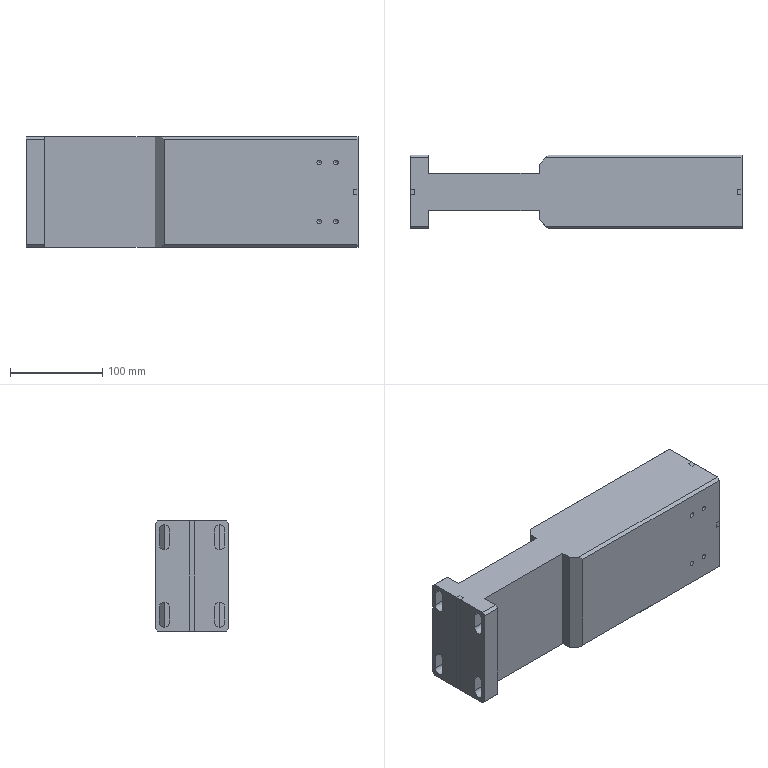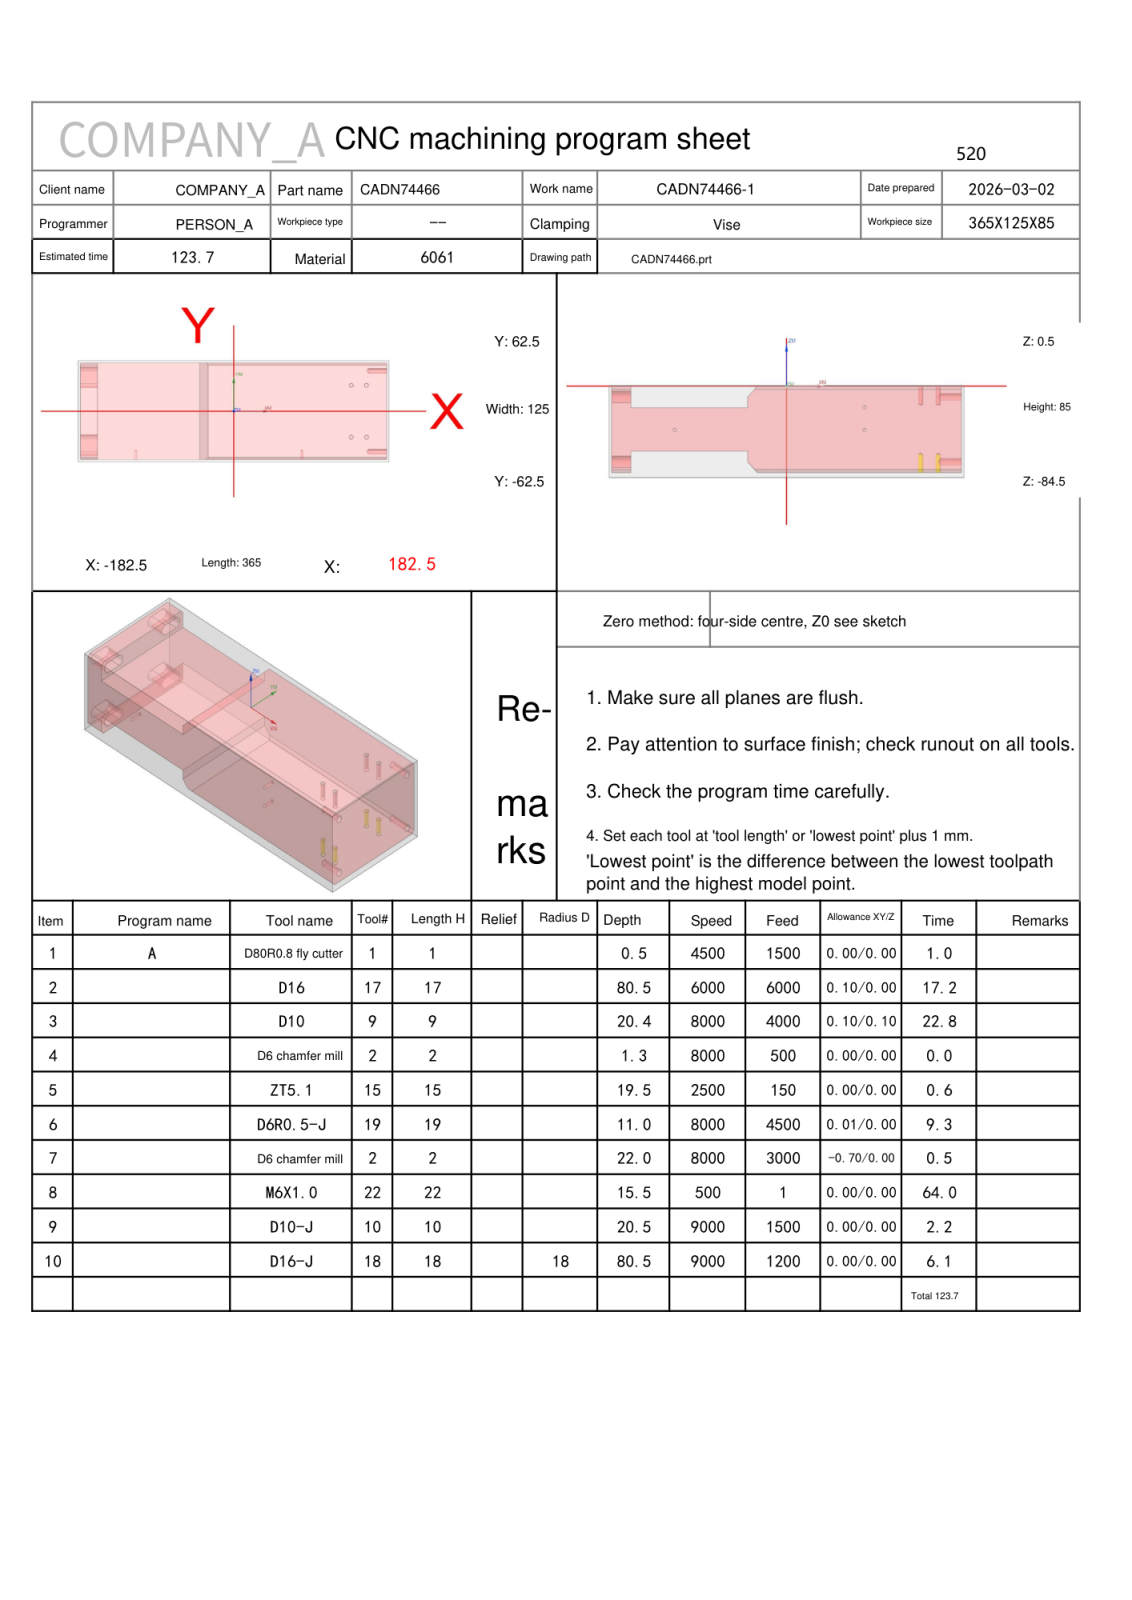NC program | NX | posted by the shop | part box 360 x 80 x 120 mm
Lines 872 to 2006 of 7747:
N3 T09 M06
(D10  D=10. R=0. H=09 ce=0.10 di=0.10)
G00 G90 G54 X-88.269 Y-74.5 M03 S8000
G43 H09 Z10.5
M08
Z.703
G01 Z-.498 F4000.
Y-67.08
G03 X-95.269 Y-60.08 I-7. J0.0
G01 X-147.9
X-154.696
X-154.901 Y-60.079
X-154.986 Y-60.083
X-154.98 Y-59.999
X-154.981 Y-58.427
G03 X-154.9 Y-57.518 I-5.04 J.908
G01 Y-57.497
Y57.497
Y57.518
G03 X-154.981 Y58.427 I-5.121 J0.0
G01 X-154.98 Y59.999
X-154.986 Y60.083
X-154.901 Y60.079
X-154.695 Y60.08
X-45.903
X-45.011
X-38.071
X-38.014 Y60.056
X-35.638 Y57.679
X-35.639 Y53.08
Y-53.08
X-35.638 Y-57.679
X-38.014 Y-60.056
X-38.071 Y-60.08
X-42.639
X-45.088
X-45.903
X-92.255
G02 X-93.068 Y-59.662 I.001 J1.
G01 X-97.471 Y-53.498
G03 X-98.284 Y-53.08 I-.813 J-.582
G01 X-146.902
G02 X-147.9 Y-52.082 I.002 J1.
G01 Y52.082
G02 X-146.902 Y53.08 I1. J-.002
G01 X-45.904
X-45.013
X-43.637
G02 X-42.639 Y52.082 I-.002 J-1.
G01 Y-52.082
G02 X-43.637 Y-53.08 I-1. J.002
G01 X-45.076
X-45.905
X-92.255
G02 X-93.068 Y-52.662 I.001 J1.
G01 X-97.471 Y-46.498
G03 X-98.284 Y-46.08 I-.813 J-.582
G01 X-139.903
G02 X-140.9 Y-45.083 I.003 J1.
G01 Y45.083
G02 X-139.903 Y46.08 I1. J-.003
G01 X-50.636
G02 X-49.639 Y45.083 I-.003 J-1.
G01 Y-45.083
G02 X-50.636 Y-46.08 I-1. J.003
G01 X-92.255
G02 X-93.068 Y-45.662 I.001 J1.
G01 X-97.471 Y-39.498
G03 X-98.284 Y-39.08 I-.813 J-.582
G01 X-132.903
G02 X-133.9 Y-38.083 I.003 J1.
G01 Y38.083
G02 X-132.903 Y39.08 I1. J-.003
G01 X-57.636
G02 X-56.639 Y38.083 I-.003 J-1.
G01 Y-38.083
G02 X-57.636 Y-39.08 I-1. J.003
G01 X-92.255
G02 X-93.068 Y-38.662 I0.0 J1.
G01 X-97.471 Y-32.498
G03 X-98.284 Y-32.08 I-.813 J-.582
G01 X-125.903
G02 X-126.9 Y-31.083 I.003 J1.
G01 Y31.083
G02 X-125.903 Y32.08 I1. J-.003
G01 X-64.636
G02 X-63.639 Y31.083 I-.003 J-1.
G01 Y-31.083
G02 X-64.636 Y-32.08 I-1. J.003
G01 X-92.255
G02 X-93.068 Y-31.662 I0.0 J1.
G01 X-97.471 Y-25.498
G03 X-98.284 Y-25.08 I-.814 J-.582
G01 X-118.904
G02 X-119.9 Y-24.084 I.004 J1.
G01 Y24.084
G02 X-118.904 Y25.08 I1. J-.004
G01 X-71.635
G02 X-70.639 Y24.084 I-.004 J-1.
G01 Y-24.084
G02 X-71.635 Y-25.08 I-1. J.004
G01 X-92.255
G02 X-93.068 Y-24.662 I0.0 J1.
G01 X-97.471 Y-18.498
G03 X-98.284 Y-18.08 I-.814 J-.582
G01 X-111.904
G02 X-112.9 Y-17.084 I.004 J1.
G01 Y17.084
G02 X-111.904 Y18.08 I1. J-.004
G01 X-78.635
G02 X-77.639 Y17.084 I-.004 J-1.
G01 Y-17.084
G02 X-78.635 Y-18.08 I-1. J.004
G01 X-92.255
G02 X-93.068 Y-17.662 I0.0 J1.
G01 X-97.471 Y-11.498
G03 X-98.284 Y-11.08 I-.814 J-.582
G01 X-104.904
G02 X-105.9 Y-10.084 I.004 J1.
G01 Y10.084
G02 X-104.904 Y11.08 I1. J-.004
G01 X-85.635
G02 X-84.639 Y10.084 I-.004 J-1.
G01 Y-10.084
G02 X-85.635 Y-11.08 I-1. J.004
G01 X-92.255
G02 X-93.068 Y-10.662 I0.0 J1.
G01 X-97.502 Y-4.455
G03 X-98.107 Y-4.058 I-.814 J-.582
G02 X-98.9 Y-3.084 I.207 J.978
G01 Y3.084
G02 X-97.904 Y4.08 I1. J-.004
G01 X-92.635
G02 X-91.639 Y3.084 I-.004 J-1.
G01 Y-3.084
G02 X-92.635 Y-4.08 I-1. J.004
G01 X-95.269
X-95.769
G03 X-102.769 Y-11.08 I0.0 J-7.
G01 Z.703
G00 Z3.
G01 X-88.269 Y-74.5 F6000.
G00 Z.205
G01 Z-.995 F4000.
Y-67.08
G03 X-95.269 Y-60.08 I-7. J0.0
G01 X-147.9
X-154.696
X-154.901 Y-60.079
X-154.986 Y-60.083
X-154.98 Y-59.999
X-154.981 Y-58.923
G03 X-154.9 Y-58.016 I-5.04 J.907
G01 Y-57.995
Y57.995
Y58.016
G03 X-154.981 Y58.923 I-5.121 J0.0
G01 X-154.98 Y59.999
X-154.986 Y60.083
X-154.901 Y60.079
X-154.695 Y60.08
X-45.903
X-45.011
X-38.071
X-38.014 Y60.056
X-36.135 Y58.177
X-36.136 Y53.08
Y-53.08
X-36.135 Y-58.177
X-38.014 Y-60.056
X-38.071 Y-60.08
X-43.136
X-45.088
X-45.903
X-92.255
G02 X-93.068 Y-59.662 I.001 J1.
G01 X-97.471 Y-53.498
G03 X-98.284 Y-53.08 I-.813 J-.582
G01 X-146.903
G02 X-147.9 Y-52.083 I.003 J1.
G01 Y52.083
G02 X-146.903 Y53.08 I1. J-.003
G01 X-45.904
X-45.013
X-44.134
G02 X-43.136 Y52.082 I-.003 J-1.
G01 Y-52.082
G02 X-44.134 Y-53.08 I-1. J.003
G01 X-45.076
X-45.905
X-92.255
G02 X-93.068 Y-52.662 I.001 J1.
G01 X-97.471 Y-46.498
G03 X-98.284 Y-46.08 I-.813 J-.582
G01 X-139.903
G02 X-140.9 Y-45.083 I.003 J1.
G01 Y45.083
G02 X-139.903 Y46.08 I1. J-.003
G01 X-51.133
G02 X-50.136 Y45.083 I-.003 J-1.
G01 Y-45.083
G02 X-51.133 Y-46.08 I-1. J.003
G01 X-92.255
G02 X-93.068 Y-45.662 I.001 J1.
G01 X-97.471 Y-39.498
G03 X-98.284 Y-39.08 I-.813 J-.582
G01 X-132.903
G02 X-133.9 Y-38.083 I.003 J1.
G01 Y38.083
G02 X-132.903 Y39.08 I1. J-.003
G01 X-58.133
G02 X-57.136 Y38.083 I-.003 J-1.
G01 Y-38.083
G02 X-58.133 Y-39.08 I-1. J.003
G01 X-92.255
G02 X-93.068 Y-38.662 I0.0 J1.
G01 X-97.471 Y-32.498
G03 X-98.284 Y-32.08 I-.813 J-.582
G01 X-125.904
G02 X-126.9 Y-31.084 I.004 J1.
G01 Y31.084
G02 X-125.904 Y32.08 I1. J-.004
G01 X-65.133
G02 X-64.136 Y31.084 I-.004 J-1.
G01 Y-31.084
G02 X-65.133 Y-32.08 I-1. J.004
G01 X-92.255
G02 X-93.068 Y-31.662 I0.0 J1.
G01 X-97.471 Y-25.498
G03 X-98.284 Y-25.08 I-.814 J-.582
G01 X-118.904
G02 X-119.9 Y-24.084 I.004 J1.
G01 Y24.084
G02 X-118.904 Y25.08 I1. J-.004
G01 X-72.133
G02 X-71.136 Y24.084 I-.004 J-1.
G01 Y-24.084
G02 X-72.133 Y-25.08 I-1. J.004
G01 X-92.255
G02 X-93.068 Y-24.662 I0.0 J1.
G01 X-97.471 Y-18.498
G03 X-98.284 Y-18.08 I-.814 J-.582
G01 X-111.904
G02 X-112.9 Y-17.084 I.004 J1.
G01 Y17.084
G02 X-111.904 Y18.08 I1. J-.004
G01 X-79.133
G02 X-78.136 Y17.084 I-.004 J-1.
G01 Y-17.084
G02 X-79.133 Y-18.08 I-1. J.004
G01 X-92.255
G02 X-93.068 Y-17.662 I0.0 J1.
G01 X-97.471 Y-11.499
G03 X-98.284 Y-11.08 I-.814 J-.581
G01 X-104.904
G02 X-105.9 Y-10.084 I.004 J1.
G01 Y10.084
G02 X-104.904 Y11.08 I1. J-.004
G01 X-86.132
G02 X-85.136 Y10.084 I-.004 J-1.
G01 Y-10.084
G02 X-86.132 Y-11.08 I-1. J.004
G01 X-92.255
G02 X-93.068 Y-10.661 I0.0 J1.
G01 X-97.502 Y-4.455
G03 X-98.107 Y-4.058 I-.814 J-.582
G02 X-98.9 Y-3.084 I.207 J.978
G01 Y3.084
G02 X-97.904 Y4.08 I1. J-.004
G01 X-93.132
G02 X-92.136 Y3.084 I-.004 J-1.
G01 Y-3.084
G02 X-93.132 Y-4.08 I-1. J.004
G01 X-95.269
X-95.769
G03 X-102.769 Y-11.08 I0.0 J-7.
G01 Z.205
G00 Z3.
G01 X-88.269 Y-74.5 F6000.
G00 Z-.293
G01 Z-1.493 F4000.
Y-67.08
G03 X-95.269 Y-60.08 I-7. J0.0
G01 X-147.9
X-154.696
X-154.901 Y-60.079
X-154.986 Y-60.083
X-154.98 Y-59.999
X-154.981 Y-59.419
G03 X-154.9 Y-58.513 I-5.04 J.906
G01 Y-58.492
Y58.492
Y58.513
G03 X-154.981 Y59.419 I-5.121 J0.0
G01 X-154.98 Y59.999
X-154.986 Y60.083
X-154.901 Y60.079
X-154.695 Y60.08
X-45.903
X-45.011
X-38.071
X-38.014 Y60.056
X-36.633 Y58.675
X-36.634 Y53.08
Y-53.08
X-36.633 Y-58.675
X-38.014 Y-60.056
X-38.071 Y-60.08
X-43.634
X-45.088
X-45.903
X-92.255
G02 X-93.068 Y-59.662 I.001 J1.
G01 X-97.471 Y-53.498
G03 X-98.284 Y-53.08 I-.813 J-.582
G01 X-146.903
G02 X-147.9 Y-52.083 I.003 J1.
G01 Y52.083
G02 X-146.903 Y53.08 I1. J-.003
G01 X-45.904
X-45.013
X-44.631
G02 X-43.634 Y52.083 I-.003 J-1.
G01 Y-52.083
G02 X-44.631 Y-53.08 I-1. J.003
G01 X-45.076
X-45.905
X-92.255
G02 X-93.068 Y-52.662 I.001 J1.
G01 X-97.471 Y-46.498
G03 X-98.284 Y-46.08 I-.813 J-.582
G01 X-139.903
G02 X-140.9 Y-45.083 I.003 J1.
G01 Y45.083
G02 X-139.903 Y46.08 I1. J-.003
G01 X-51.631
G02 X-50.634 Y45.083 I-.003 J-1.
G01 Y-45.083
G02 X-51.631 Y-46.08 I-1. J.003
G01 X-92.255
G02 X-93.068 Y-45.662 I.001 J1.
G01 X-97.471 Y-39.498
G03 X-98.284 Y-39.08 I-.813 J-.582
G01 X-132.904
G02 X-133.9 Y-38.084 I.004 J1.
G01 Y38.084
G02 X-132.904 Y39.08 I1. J-.004
G01 X-58.63
G02 X-57.634 Y38.084 I-.004 J-1.
G01 Y-38.084
G02 X-58.63 Y-39.08 I-1. J.004
G01 X-92.255
G02 X-93.068 Y-38.662 I0.0 J1.
G01 X-97.471 Y-32.498
G03 X-98.284 Y-32.08 I-.813 J-.582
G01 X-125.904
G02 X-126.9 Y-31.084 I.004 J1.
G01 Y31.084
G02 X-125.904 Y32.08 I1. J-.004
G01 X-65.63
G02 X-64.634 Y31.084 I-.004 J-1.
G01 Y-31.084
G02 X-65.63 Y-32.08 I-1. J.004
G01 X-92.255
G02 X-93.068 Y-31.662 I0.0 J1.
G01 X-97.471 Y-25.498
G03 X-98.284 Y-25.08 I-.814 J-.582
G01 X-118.904
G02 X-119.9 Y-24.084 I.004 J1.
G01 Y24.084
G02 X-118.904 Y25.08 I1. J-.004
G01 X-72.63
G02 X-71.634 Y24.084 I-.004 J-1.
G01 Y-24.084
G02 X-72.63 Y-25.08 I-1. J.004
G01 X-92.255
G02 X-93.068 Y-24.662 I0.0 J1.
G01 X-97.471 Y-18.498
G03 X-98.284 Y-18.08 I-.814 J-.582
G01 X-111.904
G02 X-112.9 Y-17.084 I.004 J1.
G01 Y17.084
G02 X-111.904 Y18.08 I1. J-.004
G01 X-79.63
G02 X-78.634 Y17.084 I-.004 J-1.
G01 Y-17.084
G02 X-79.63 Y-18.08 I-1. J.004
G01 X-92.255
G02 X-93.068 Y-17.662 I0.0 J1.
G01 X-97.471 Y-11.499
G03 X-98.284 Y-11.08 I-.814 J-.581
G01 X-104.904
G02 X-105.9 Y-10.084 I.004 J1.
G01 Y10.084
G02 X-104.904 Y11.08 I1. J-.004
G01 X-86.63
G02 X-85.634 Y10.084 I-.004 J-1.
G01 Y-10.084
G02 X-86.63 Y-11.08 I-1. J.004
G01 X-92.255
G02 X-93.068 Y-10.661 I0.0 J1.
G01 X-97.502 Y-4.455
G03 X-98.107 Y-4.058 I-.814 J-.582
G02 X-98.9 Y-3.084 I.207 J.978
G01 Y3.084
G02 X-97.904 Y4.08 I1. J-.004
G01 X-93.63
G02 X-92.634 Y3.084 I-.004 J-1.
G01 Y-3.084
G02 X-93.63 Y-4.08 I-1. J.004
G01 X-95.269
X-95.769
G03 X-102.769 Y-11.08 I0.0 J-7.
G01 Z-.293
G00 Z3.
G01 X-88.269 Y-74.5 F6000.
G00 Z-.79
G01 Z-1.99 F4000.
Y-67.08
G03 X-95.269 Y-60.08 I-7. J0.0
G01 X-147.9
X-154.696
X-154.901 Y-60.079
X-154.986 Y-60.083
X-154.98 Y-59.999
Y-59.902
G03 X-154.9 Y-58.996 I-5.055 J.906
G01 Y-58.99
Y58.99
Y59.011
G03 X-154.98 Y59.915 I-5.121 J0.0
G01 Y59.999
X-154.986 Y60.083
X-154.901 Y60.079
X-154.695 Y60.08
X-45.903
X-45.011
X-38.071
X-38.014 Y60.056
X-37.13 Y59.172
X-37.131 Y53.08
Y-53.076
X-37.13 Y-59.172
X-38.014 Y-60.056
X-38.071 Y-60.08
X-44.131
X-45.088
X-45.903
X-92.255
G02 X-93.068 Y-59.662 I.001 J1.
G01 X-97.471 Y-53.498
G03 X-98.284 Y-53.08 I-.813 J-.582
G01 X-146.903
G02 X-147.9 Y-52.083 I.003 J1.
G01 Y52.083
G02 X-146.903 Y53.08 I1. J-.003
G01 X-45.904
X-45.128
G02 X-44.131 Y52.083 I-.003 J-1.
G01 Y-52.083
G02 X-45.128 Y-53.08 I-1. J.003
G01 X-45.905
X-92.255
G02 X-93.068 Y-52.662 I.001 J1.
G01 X-97.471 Y-46.498
G03 X-98.284 Y-46.08 I-.813 J-.582
G01 X-139.903
G02 X-140.9 Y-45.083 I.003 J1.
G01 Y45.083
G02 X-139.903 Y46.08 I1. J-.003
G01 X-52.128
G02 X-51.131 Y45.083 I-.003 J-1.
G01 Y-45.083
G02 X-52.128 Y-46.08 I-1. J.003
G01 X-92.255
G02 X-93.068 Y-45.662 I.001 J1.
G01 X-97.471 Y-39.498
G03 X-98.284 Y-39.08 I-.813 J-.582
G01 X-132.904
G02 X-133.9 Y-38.084 I.004 J1.
G01 Y38.084
G02 X-132.904 Y39.08 I1. J-.004
G01 X-59.128
G02 X-58.131 Y38.084 I-.004 J-1.
G01 Y-38.084
G02 X-59.128 Y-39.08 I-1. J.004
G01 X-92.255
G02 X-93.068 Y-38.662 I0.0 J1.
G01 X-97.471 Y-32.498
G03 X-98.284 Y-32.08 I-.813 J-.582
G01 X-125.904
G02 X-126.9 Y-31.084 I.004 J1.
G01 Y31.084
G02 X-125.904 Y32.08 I1. J-.004
G01 X-66.127
G02 X-65.131 Y31.084 I-.004 J-1.
G01 Y-31.084
G02 X-66.127 Y-32.08 I-1. J.004
G01 X-92.255
G02 X-93.068 Y-31.662 I0.0 J1.
G01 X-97.471 Y-25.498
G03 X-98.284 Y-25.08 I-.813 J-.582
G01 X-118.904
G02 X-119.9 Y-24.084 I.004 J1.
G01 Y24.084
G02 X-118.904 Y25.08 I1. J-.004
G01 X-73.127
G02 X-72.131 Y24.084 I-.004 J-1.
G01 Y-24.084
G02 X-73.127 Y-25.08 I-1. J.004
G01 X-92.255
G02 X-93.068 Y-24.662 I0.0 J1.
G01 X-97.471 Y-18.498
G03 X-98.284 Y-18.08 I-.814 J-.582
G01 X-111.904
G02 X-112.9 Y-17.084 I.004 J1.
G01 Y17.084
G02 X-111.904 Y18.08 I1. J-.004
G01 X-80.127
G02 X-79.131 Y17.084 I-.004 J-1.
G01 Y-17.084
G02 X-80.127 Y-18.08 I-1. J.004
G01 X-92.255
G02 X-93.068 Y-17.662 I0.0 J1.
G01 X-97.471 Y-11.499
G03 X-98.284 Y-11.08 I-.814 J-.581
G01 X-104.904
G02 X-105.9 Y-10.084 I.004 J1.
G01 Y10.084
G02 X-104.904 Y11.08 I1. J-.004
G01 X-87.127
G02 X-86.131 Y10.084 I-.004 J-1.
G01 Y-10.084
G02 X-87.127 Y-11.08 I-1. J.004
G01 X-92.255
G02 X-93.068 Y-10.661 I0.0 J1.
G01 X-97.502 Y-4.455
G03 X-98.107 Y-4.058 I-.814 J-.582
G02 X-98.9 Y-3.084 I.207 J.978
G01 Y3.084
G02 X-97.904 Y4.08 I1. J-.004
G01 X-94.127
G02 X-93.131 Y3.084 I-.004 J-1.
G01 Y-3.084
G02 X-94.127 Y-4.08 I-1. J.004
G01 X-95.269
X-95.769
G03 X-102.769 Y-11.08 I0.0 J-7.
G01 Z-.79
G00 Z3.
G01 X-88.269 Y-74.5 F6000.
G00 Z-1.288
G01 Z-2.488 F4000.
Y-67.08
G03 X-95.269 Y-60.08 I-7. J0.0
G01 X-147.9
X-154.696
X-154.901 Y-60.079
X-154.932 Y-60.072
G03 X-154.9 Y-59.496 I-5.1 J.576
G01 Y-59.487
Y59.487
Y59.496
G03 X-154.932 Y60.072 I-5.133 J0.0
G01 X-154.901 Y60.079
X-154.695 Y60.08
X-45.903
X-45.011
X-38.071
X-38.014 Y60.056
X-37.628 Y59.67
X-37.629 Y53.08
Y-53.076
X-37.628 Y-59.67
X-38.014 Y-60.056
X-38.071 Y-60.08
X-44.629
X-45.088
X-45.903
X-92.255
G02 X-93.068 Y-59.662 I.001 J1.
G01 X-97.471 Y-53.498
G03 X-98.284 Y-53.08 I-.813 J-.582
G01 X-146.903
G02 X-147.9 Y-52.083 I.003 J1.
G01 Y52.083
G02 X-146.903 Y53.08 I1. J-.003
G01 X-45.904
X-45.626
G02 X-44.629 Y52.083 I-.003 J-1.
G01 Y-52.083
G02 X-45.625 Y-53.08 I-1. J.003
G01 X-45.905
X-92.255
G02 X-93.068 Y-52.662 I.001 J1.
G01 X-97.471 Y-46.498
G03 X-98.284 Y-46.08 I-.813 J-.582
G01 X-139.904
G02 X-140.9 Y-45.084 I.004 J1.
G01 Y45.084
G02 X-139.904 Y46.08 I1. J-.004
G01 X-52.625
G02 X-51.629 Y45.084 I-.004 J-1.
G01 Y-45.084
G02 X-52.625 Y-46.08 I-1. J.004
G01 X-92.255
G02 X-93.068 Y-45.662 I.001 J1.
G01 X-97.471 Y-39.498
G03 X-98.284 Y-39.08 I-.813 J-.582
G01 X-132.904
G02 X-133.9 Y-38.084 I.004 J1.
G01 Y38.084
G02 X-132.904 Y39.08 I1. J-.004
G01 X-59.625
G02 X-58.629 Y38.084 I-.004 J-1.
G01 Y-38.084
G02 X-59.625 Y-39.08 I-1. J.004
G01 X-92.255
G02 X-93.068 Y-38.662 I0.0 J1.
G01 X-97.471 Y-32.498
G03 X-98.284 Y-32.08 I-.813 J-.582
G01 X-125.904
G02 X-126.9 Y-31.084 I.004 J1.
G01 Y31.084
G02 X-125.904 Y32.08 I1. J-.004
G01 X-66.625
G02 X-65.629 Y31.084 I-.004 J-1.
G01 Y-31.084
G02 X-66.625 Y-32.08 I-1. J.004
G01 X-92.255
G02 X-93.068 Y-31.662 I0.0 J1.
G01 X-97.471 Y-25.498
G03 X-98.284 Y-25.08 I-.814 J-.582
G01 X-118.904
G02 X-119.9 Y-24.084 I.004 J1.
G01 Y24.084
G02 X-118.904 Y25.08 I1. J-.004
G01 X-73.625
G02 X-72.629 Y24.084 I-.004 J-1.
G01 Y-24.084
G02 X-73.625 Y-25.08 I-1. J.004
G01 X-92.255
G02 X-93.068 Y-24.662 I0.0 J1.
G01 X-97.471 Y-18.498
G03 X-98.284 Y-18.08 I-.814 J-.582
G01 X-111.904
G02 X-112.9 Y-17.084 I.004 J1.
G01 Y17.084
G02 X-111.904 Y18.08 I1. J-.004
G01 X-80.624
G02 X-79.629 Y17.084 I-.004 J-1.
G01 Y-17.084
G02 X-80.624 Y-18.08 I-1. J.004
G01 X-92.255
G02 X-93.068 Y-17.662 I0.0 J1.
G01 X-97.471 Y-11.499
G03 X-98.284 Y-11.08 I-.814 J-.581
G01 X-104.905
G02 X-105.9 Y-10.085 I.005 J1.
G01 Y10.085
G02 X-104.905 Y11.08 I1. J-.005
G01 X-87.624
G02 X-86.629 Y10.085 I-.005 J-1.
G01 Y-10.085
G02 X-87.624 Y-11.08 I-1. J.005
G01 X-92.255
G02 X-93.068 Y-10.661 I0.0 J1.
G01 X-97.502 Y-4.455
G03 X-98.107 Y-4.058 I-.814 J-.582
G02 X-98.9 Y-3.085 I.207 J.978
G01 Y3.085
G02 X-97.905 Y4.08 I1. J-.005
G01 X-94.624
G02 X-93.629 Y3.085 I-.005 J-1.
G01 Y-3.085
G02 X-94.624 Y-4.08 I-1. J.005
G01 X-95.269
X-95.769
G03 X-102.769 Y-11.08 I0.0 J-7.
G01 Z-1.288
G00 Z3.
G01 X-88.269 Y-74.5 F6000.
G00 Z-1.785
G01 Z-2.985 F4000.
Y-67.08
G03 X-95.269 Y-60.08 I-7. J0.0
G01 X-147.9
X-154.696
X-154.901 Y-60.079
X-154.9 Y-59.488
X-154.901 Y60.079
X-154.695 Y60.08
X-45.903
X-45.011
X-38.125
X-38.126 Y53.08
Y-53.08
X-38.125 Y-60.08
X-45.126
X-45.903
X-92.255
G02 X-93.068 Y-59.662 I.001 J1.
G01 X-97.471 Y-53.498
G03 X-98.284 Y-53.08 I-.813 J-.582
G01 X-146.904
G02 X-147.9 Y-52.084 I.004 J1.
G01 Y52.084
G02 X-146.904 Y53.08 I1. J-.004
G01 X-46.123
G02 X-45.126 Y52.084 I-.004 J-1.
G01 Y-52.084
G02 X-46.123 Y-53.08 I-1. J.004
G01 X-92.255
G02 X-93.068 Y-52.662 I.001 J1.
G01 X-97.471 Y-46.498
G03 X-98.284 Y-46.08 I-.813 J-.582
G01 X-139.904
G02 X-140.9 Y-45.084 I.004 J1.
G01 Y45.084
G02 X-139.904 Y46.08 I1. J-.004
G01 X-53.123
G02 X-52.126 Y45.084 I-.004 J-1.
G01 Y-45.084
G02 X-53.123 Y-46.08 I-1. J.004
G01 X-92.255
G02 X-93.068 Y-45.662 I.001 J1.
G01 X-97.471 Y-39.498
G03 X-98.284 Y-39.08 I-.813 J-.582
G01 X-132.904
G02 X-133.9 Y-38.084 I.004 J1.
G01 Y38.084
G02 X-132.904 Y39.08 I1. J-.004
G01 X-60.122
G02 X-59.126 Y38.084 I-.004 J-1.
G01 Y-38.084
G02 X-60.122 Y-39.08 I-1. J.004
G01 X-92.255
G02 X-93.068 Y-38.662 I0.0 J1.
G01 X-97.471 Y-32.498
G03 X-98.284 Y-32.08 I-.813 J-.582
G01 X-125.904
G02 X-126.9 Y-31.084 I.004 J1.
G01 Y31.084
G02 X-125.904 Y32.08 I1. J-.004
G01 X-67.122
G02 X-66.126 Y31.084 I-.004 J-1.
G01 Y-31.084
G02 X-67.122 Y-32.08 I-1. J.004
G01 X-92.255
G02 X-93.068 Y-31.662 I0.0 J1.
G01 X-97.471 Y-25.498
G03 X-98.284 Y-25.08 I-.814 J-.582
G01 X-118.904
G02 X-119.9 Y-24.084 I.004 J1.
G01 Y24.084
G02 X-118.904 Y25.08 I1. J-.004
G01 X-74.122
G02 X-73.126 Y24.084 I-.004 J-1.
G01 Y-24.084
G02 X-74.122 Y-25.08 I-1. J.004
G01 X-92.255
G02 X-93.068 Y-24.662 I0.0 J1.
G01 X-97.471 Y-18.498
G03 X-98.284 Y-18.08 I-.814 J-.582
G01 X-111.905
G02 X-112.9 Y-17.085 I.005 J1.
G01 Y17.085
G02 X-111.905 Y18.08 I1. J-.005
G01 X-81.122
G02 X-80.126 Y17.085 I-.005 J-1.
G01 Y-17.085
G02 X-81.122 Y-18.08 I-1. J.005
G01 X-92.255
G02 X-93.068 Y-17.662 I0.0 J1.
G01 X-97.471 Y-11.499
G03 X-98.284 Y-11.08 I-.814 J-.581
G01 X-104.905
G02 X-105.9 Y-10.085 I.005 J1.
G01 Y10.085
G02 X-104.905 Y11.08 I1. J-.005
G01 X-88.122
G02 X-87.126 Y10.085 I-.005 J-1.
G01 Y-10.085
G02 X-88.122 Y-11.08 I-1. J.005
G01 X-92.255
G02 X-93.068 Y-10.661 I0.0 J1.
G01 X-97.502 Y-4.455
G03 X-98.107 Y-4.058 I-.814 J-.582
G02 X-98.9 Y-3.085 I.207 J.978
G01 Y3.085
G02 X-97.905 Y4.08 I1. J-.005
G01 X-95.122
G02 X-94.126 Y3.085 I-.005 J-1.
G01 Y-3.085
G02 X-95.122 Y-4.08 I-1. J.005
G01 X-95.269
X-95.769
G03 X-102.769 Y-11.08 I0.0 J-7.
G01 Z-1.785
G00 Z3.
G01 X-88.269 Y-74.5 F6000.
G00 Z-2.283
G01 Z-3.483 F4000.
Y-67.08
G03 X-95.269 Y-60.08 I-7. J0.0
G01 X-147.9
X-154.696
X-154.901 Y-60.079
X-154.9 Y-53.08
Y53.08
X-154.901 Y60.079
X-154.695 Y60.08
X-45.903
X-45.624
X-45.011
X-38.623
X-38.624 Y53.08
Y-53.08
X-38.623 Y-60.08
X-45.088
X-45.903
X-92.255
G02 X-93.068 Y-59.662 I.001 J1.
G01 X-97.471 Y-53.498
G03 X-98.284 Y-53.08 I-.813 J-.582
G01 X-146.904
G02 X-147.9 Y-52.084 I.004 J1.
G01 Y52.084
G02 X-146.904 Y53.08 I1. J-.004
G01 X-46.62
G02 X-45.624 Y52.084 I-.004 J-1.
G01 Y-52.084
G02 X-46.62 Y-53.08 I-1. J.004
G01 X-92.255
G02 X-93.068 Y-52.662 I.001 J1.
G01 X-97.471 Y-46.498
G03 X-98.284 Y-46.08 I-.813 J-.582
G01 X-139.904
G02 X-140.9 Y-45.084 I.004 J1.
G01 Y45.084
G02 X-139.904 Y46.08 I1. J-.004
G01 X-53.62
G02 X-52.624 Y45.084 I-.004 J-1.
G01 Y-45.084
G02 X-53.62 Y-46.08 I-1. J.004
G01 X-92.255
G02 X-93.068 Y-45.662 I0.0 J1.
G01 X-97.471 Y-39.498
G03 X-98.284 Y-39.08 I-.813 J-.582
G01 X-132.904
G02 X-133.9 Y-38.084 I.004 J1.
G01 Y38.084
G02 X-132.904 Y39.08 I1. J-.004
G01 X-60.62
G02 X-59.624 Y38.084 I-.004 J-1.
G01 Y-38.084
G02 X-60.62 Y-39.08 I-1. J.004
G01 X-92.255
G02 X-93.068 Y-38.662 I0.0 J1.
G01 X-97.471 Y-32.498
G03 X-98.284 Y-32.08 I-.813 J-.582
G01 X-125.904
G02 X-126.9 Y-31.084 I.004 J1.
G01 Y31.084
G02 X-125.904 Y32.08 I1. J-.004
G01 X-67.619
G02 X-66.624 Y31.084 I-.004 J-1.
G01 Y-31.084
G02 X-67.619 Y-32.08 I-1. J.004
G01 X-92.255
G02 X-93.068 Y-31.662 I0.0 J1.
G01 X-97.471 Y-25.498
G03 X-98.284 Y-25.08 I-.814 J-.582
G01 X-118.905
G02 X-119.9 Y-24.085 I.005 J1.
G01 Y24.085
G02 X-118.905 Y25.08 I1. J-.005
G01 X-74.619
G02 X-73.624 Y24.085 I-.005 J-1.
G01 Y-24.085
G02 X-74.619 Y-25.08 I-1. J.005
G01 X-92.255
G02 X-93.068 Y-24.662 I0.0 J1.
G01 X-97.471 Y-18.498
G03 X-98.284 Y-18.08 I-.814 J-.582
G01 X-111.905
G02 X-112.9 Y-17.085 I.005 J1.
G01 Y17.085
G02 X-111.905 Y18.08 I1. J-.005
G01 X-81.619
G02 X-80.624 Y17.085 I-.005 J-1.
G01 Y-17.085
G02 X-81.619 Y-18.08 I-1. J.005
G01 X-92.255
G02 X-93.068 Y-17.662 I0.0 J1.
G01 X-97.471 Y-11.498
G03 X-98.284 Y-11.08 I-.814 J-.582
G01 X-104.905
G02 X-105.9 Y-10.085 I.005 J1.
G01 Y10.085
G02 X-104.905 Y11.08 I1. J-.005
G01 X-88.619
G02 X-87.624 Y10.085 I-.005 J-1.
G01 Y-10.085
G02 X-88.619 Y-11.08 I-1. J.005
G01 X-92.272
G02 X-93.069 Y-10.684 I0.0 J1.
G01 X-97.888 Y-4.316
G03 X-98.292 Y-4. I-.797 J-.604
G02 X-98.9 Y-3.085 I.392 J.92
G01 Y3.085
G02 X-97.905 Y4.08 I1. J-.005
G01 X-95.619
G02 X-94.624 Y3.085 I-.005 J-1.
G01 Y-3.085
G02 X-95.58 Y-4.079 I-1. J.005
G01 X-96.08 Y-4.08
G03 X-103.08 Y-11.08 I0.0 J-7.
G01 Z-2.283
G00 Z3.
G01 X-88.269 Y-74.5 F6000.
G00 Z-2.78
G01 Z-3.98 F4000.
Y-67.08
G03 X-95.269 Y-60.08 I-7. J0.0
G01 X-147.9
X-154.696
X-154.901 Y-60.079
X-154.9 Y-53.08
Y53.08
X-154.901 Y60.079
X-154.695 Y60.08
X-45.903
X-45.011
X-39.12
X-39.121 Y53.08
Y-53.08
X-39.12 Y-60.08
X-45.088
X-45.903
X-92.255
G02 X-93.068 Y-59.662 I.001 J1.
G01 X-97.471 Y-53.498
G03 X-98.284 Y-53.08 I-.813 J-.582
G01 X-146.904
G02 X-147.9 Y-52.084 I.004 J1.
G01 Y52.084
G02 X-146.904 Y53.08 I1. J-.004
G01 X-47.117
G02 X-46.121 Y52.084 I-.004 J-1.
G01 Y-52.084
G02 X-47.117 Y-53.08 I-1. J.004
G01 X-92.255
G02 X-93.068 Y-52.662 I.001 J1.
G01 X-97.471 Y-46.498
G03 X-98.284 Y-46.08 I-.813 J-.582
G01 X-139.904
G02 X-140.9 Y-45.084 I.004 J1.
G01 Y45.084
G02 X-139.904 Y46.08 I1. J-.004
G01 X-54.117
G02 X-53.121 Y45.084 I-.004 J-1.
G01 Y-45.084
G02 X-54.117 Y-46.08 I-1. J.004
G01 X-92.255
G02 X-93.068 Y-45.662 I0.0 J1.
G01 X-97.471 Y-39.498
G03 X-98.284 Y-39.08 I-.813 J-.582
G01 X-132.904
G02 X-133.9 Y-38.084 I.004 J1.
G01 Y38.084
G02 X-132.904 Y39.08 I1. J-.004
G01 X-61.117
G02 X-60.121 Y38.084 I-.004 J-1.
G01 Y-38.084
G02 X-61.117 Y-39.08 I-1. J.004
G01 X-92.255
G02 X-93.068 Y-38.662 I0.0 J1.
G01 X-97.471 Y-32.498
G03 X-98.284 Y-32.08 I-.813 J-.582
G01 X-125.905
G02 X-126.9 Y-31.085 I.005 J1.
G01 Y31.085
G02 X-125.905 Y32.08 I1. J-.005
G01 X-68.117
G02 X-67.121 Y31.085 I-.005 J-1.
G01 Y-31.085
G02 X-68.117 Y-32.08 I-1. J.005
G01 X-92.255
G02 X-93.068 Y-31.662 I0.0 J1.
G01 X-97.471 Y-25.498
G03 X-98.284 Y-25.08 I-.814 J-.582
G01 X-118.905
G02 X-119.9 Y-24.085 I.005 J1.
G01 Y24.085
G02 X-118.905 Y25.08 I1. J-.005
G01 X-75.117
G02 X-74.121 Y24.085 I-.005 J-1.
G01 Y-24.085
G02 X-75.117 Y-25.08 I-1. J.005
G01 X-92.255
G02 X-93.068 Y-24.662 I0.0 J1.
G01 X-97.471 Y-18.498
G03 X-98.284 Y-18.08 I-.814 J-.582
G01 X-111.905
G02 X-112.9 Y-17.085 I.005 J1.
G01 Y17.085
G02 X-111.905 Y18.08 I1. J-.005
G01 X-82.116
G02 X-81.121 Y17.085 I-.005 J-1.
G01 Y-17.085
G02 X-82.116 Y-18.08 I-1. J.005
G01 X-92.255
G02 X-93.068 Y-17.662 I0.0 J1.
G01 X-97.471 Y-11.498
G03 X-98.284 Y-11.08 I-.814 J-.582
G01 X-104.905
G02 X-105.9 Y-10.085 I.005 J1.
G01 Y10.085
G02 X-104.905 Y11.08 I1. J-.005
G01 X-89.116
G02 X-88.121 Y10.085 I-.005 J-1.
G01 Y-10.085
G02 X-89.116 Y-11.08 I-1. J.005
G01 X-92.287
G02 X-93.07 Y-10.702 I0.0 J1.
G01 X-98.404 Y-3.989
X-98.543 Y-3.846
G02 X-98.9 Y-3.085 I.643 J.766
G01 Y3.085
G02 X-97.905 Y4.08 I1. J-.005
G01 X-96.116
G02 X-95.121 Y3.085 I-.005 J-1.
G01 Y-3.085
G02 X-96.016 Y-4.074 I-1. J.005
G01 X-96.116 Y-4.08
X-96.515
G03 X-103.515 Y-11.08 I0.0 J-7.
G01 Z-2.78
G00 Z3.
G01 X-88.269 Y-74.5 F6000.
G00 Z-3.278
G01 Z-4.478 F4000.
Y-67.08
G03 X-95.269 Y-60.08 I-7. J0.0
G01 X-147.9
X-154.696
X-154.901 Y-60.079
X-154.9 Y-53.08
Y53.08
X-154.901 Y60.079
X-154.695 Y60.08
X-45.903
X-45.011
X-39.618
X-39.619 Y53.08
Y-53.08
X-39.618 Y-60.08
X-45.088
X-45.903
X-92.255
G02 X-93.068 Y-59.662 I.001 J1.
G01 X-97.471 Y-53.498
G03 X-98.284 Y-53.08 I-.813 J-.582
G01 X-146.904
G02 X-147.9 Y-52.084 I.004 J1.
G01 Y52.084
G02 X-146.904 Y53.08 I1. J-.004
G01 X-47.615
G02 X-46.619 Y52.084 I-.004 J-1.
G01 Y-52.084
G02 X-47.615 Y-53.08 I-1. J.004
G01 X-92.255
G02 X-93.068 Y-52.662 I.001 J1.
G01 X-97.471 Y-46.498
G03 X-98.284 Y-46.08 I-.813 J-.582
G01 X-139.904
G02 X-140.9 Y-45.084 I.004 J1.
G01 Y45.084
G02 X-139.904 Y46.08 I1. J-.004
G01 X-54.614
G02 X-53.619 Y45.084 I-.004 J-1.
G01 Y-45.084
G02 X-54.614 Y-46.08 I-1. J.004
G01 X-92.255
G02 X-93.068 Y-45.662 I.001 J1.
G01 X-97.471 Y-39.498
G03 X-98.284 Y-39.08 I-.813 J-.582
G01 X-132.905
G02 X-133.9 Y-38.085 I.005 J1.
G01 Y38.085
G02 X-132.905 Y39.08 I1. J-.005
G01 X-61.614
G02 X-60.619 Y38.085 I-.005 J-1.
G01 Y-38.085
G02 X-61.614 Y-39.08 I-1. J.005
G01 X-92.255
G02 X-93.068 Y-38.662 I0.0 J1.
G01 X-97.471 Y-32.498
G03 X-98.284 Y-32.08 I-.813 J-.582
G01 X-125.905
G02 X-126.9 Y-31.085 I.005 J1.
G01 Y31.085
G02 X-125.905 Y32.08 I1. J-.005
G01 X-68.614
G02 X-67.619 Y31.085 I-.005 J-1.
G01 Y-31.085
G02 X-68.614 Y-32.08 I-1. J.005
G01 X-92.255
G02 X-93.068 Y-31.662 I0.0 J1.
G01 X-97.471 Y-25.498
G03 X-98.284 Y-25.08 I-.813 J-.582
G01 X-118.905
G02 X-119.9 Y-24.085 I.005 J1.
G01 Y24.085
G02 X-118.905 Y25.08 I1. J-.005
G01 X-75.614
G02 X-74.619 Y24.085 I-.005 J-1.
G01 Y-24.085
G02 X-75.614 Y-25.08 I-1. J.005
G01 X-92.255
G02 X-93.068 Y-24.662 I0.0 J1.
G01 X-97.471 Y-18.498
G03 X-98.284 Y-18.08 I-.814 J-.582
G01 X-111.905
G02 X-112.9 Y-17.085 I.005 J1.
G01 Y17.085
G02 X-111.905 Y18.08 I1. J-.005
G01 X-82.614
G02 X-81.619 Y17.085 I-.005 J-1.
G01 Y-17.085
G02 X-82.614 Y-18.08 I-1. J.005
G01 X-92.255
G02 X-93.068 Y-17.662 I0.0 J1.
G01 X-97.471 Y-11.499